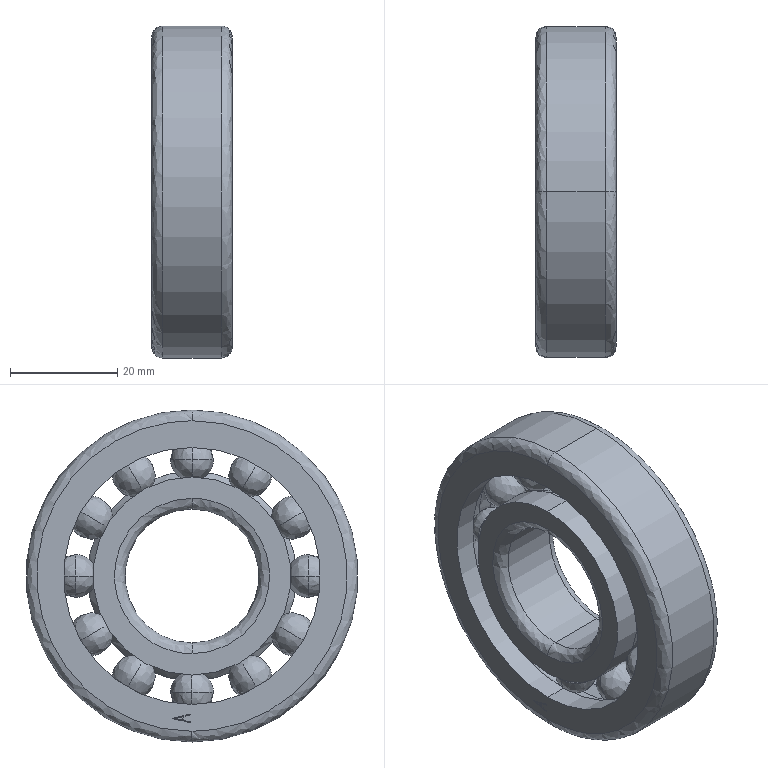Part | SolidWorks | features BaseBody 14 | 14 solids | 131 faces | box 15 x 62 x 62 mm | volume 27962 mm3 | spline 81 | plane 38 | cylinder 12 | commonest cylinder face diameters 25 x2 37 x2 39 x2 48 x2 50 x2 62 x2